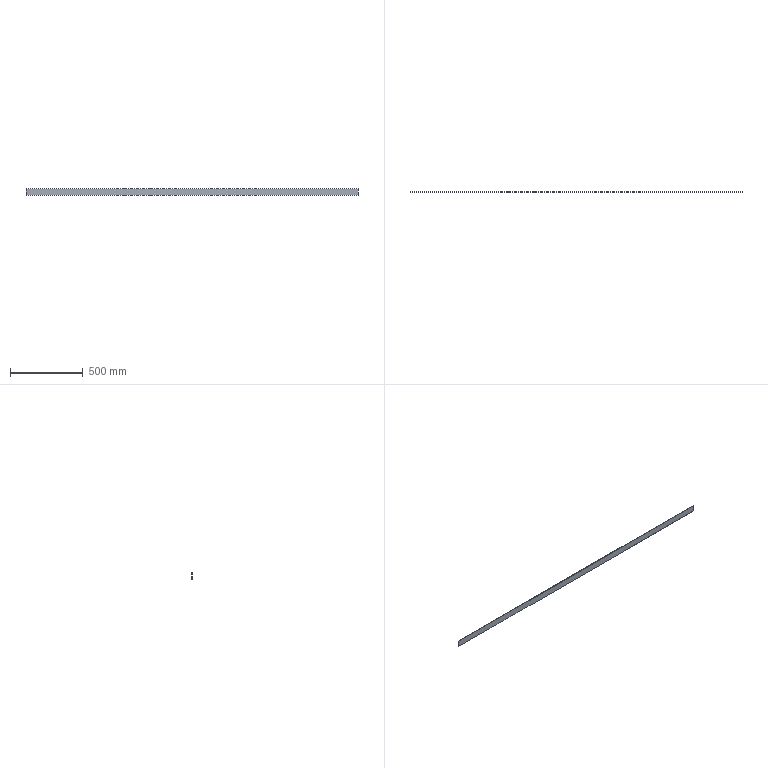Part | STEP file | SN10_017_003-01_CHAPA | 1 solid | 6 faces | box 2283 x 3 x 45 mm | volume 308205 mm3 | plane 6
STEP:
#1=CARTESIAN_POINT('',(0.,0.,0.));
#2=DIRECTION('',(0.,0.,1.));
#3=DIRECTION('',(1.,0.,0.));
#4=AXIS2_PLACEMENT_3D('',#1,#2,#3);
#5=CARTESIAN_POINT('',(3520.,-1740.,50.));
#6=VERTEX_POINT('',#5);
#7=CARTESIAN_POINT('',(1237.,-1740.,50.));
#8=VERTEX_POINT('',#7);
#9=CARTESIAN_POINT('',(3520.,-1740.,50.));
#10=DIRECTION('',(-1.,0.,0.));
#11=VECTOR('',#10,1.);
#12=LINE('',#9,#11);
#13=CARTESIAN_POINT('',(3520.,-1740.,95.));
#14=DIRECTION('',(0.,-1.,0.));
#15=DIRECTION('',(0.,0.,-1.));
#16=AXIS2_PLACEMENT_3D('',#13,#14,#15);
#17=PLANE('',#16);
#18=CARTESIAN_POINT('',(45.,0.));
#19=DIRECTION('',(0.,-1.));
#20=VECTOR('',#19,1.);
#21=LINE('',#18,#20);
#22=(GEOMETRIC_REPRESENTATION_CONTEXT(2)PARAMETRIC_REPRESENTATION_CONTEXT()REPRESENTATION_CONTEXT('',''));
#23=DEFINITIONAL_REPRESENTATION('',(#21),#22);
#24=PCURVE('',#17,#23);
#25=CARTESIAN_POINT('',(0.,0.,50.));
#26=DIRECTION('',(0.,0.,1.));
#27=DIRECTION('',(1.,0.,0.));
#28=AXIS2_PLACEMENT_3D('',#25,#26,#27);
#29=PLANE('',#28);
#30=CARTESIAN_POINT('',(3520.,-1740.));
#31=DIRECTION('',(-1.,0.));
#32=VECTOR('',#31,1.);
#33=LINE('',#30,#32);
#34=(GEOMETRIC_REPRESENTATION_CONTEXT(2)PARAMETRIC_REPRESENTATION_CONTEXT()REPRESENTATION_CONTEXT('',''));
#35=DEFINITIONAL_REPRESENTATION('',(#33),#34);
#36=PCURVE('',#29,#35);
#37=SURFACE_CURVE('',#12,(#24,#36),.PCURVE_S1.);
#38=EDGE_CURVE('',#6,#8,#37,.T.);
#39=ORIENTED_EDGE('',*,*,#38,.T.);
#40=CARTESIAN_POINT('',(1237.,-1740.,95.));
#41=VERTEX_POINT('',#40);
#42=CARTESIAN_POINT('',(1237.,-1740.,95.));
#43=DIRECTION('',(0.,0.,-1.));
#44=VECTOR('',#43,1.);
#45=LINE('',#42,#44);
#46=CARTESIAN_POINT('',(0.,-2283.));
#47=DIRECTION('',(1.,0.));
#48=VECTOR('',#47,1.);
#49=LINE('',#46,#48);
#50=(GEOMETRIC_REPRESENTATION_CONTEXT(2)PARAMETRIC_REPRESENTATION_CONTEXT()REPRESENTATION_CONTEXT('',''));
#51=DEFINITIONAL_REPRESENTATION('',(#49),#50);
#52=PCURVE('',#17,#51);
#53=CARTESIAN_POINT('',(1237.,-1740.,95.));
#54=DIRECTION('',(1.,0.,0.));
#55=DIRECTION('',(0.,0.,-1.));
#56=AXIS2_PLACEMENT_3D('',#53,#54,#55);
#57=PLANE('',#56);
#58=CARTESIAN_POINT('',(0.,0.));
#59=DIRECTION('',(1.,0.));
#60=VECTOR('',#59,1.);
#61=LINE('',#58,#60);
#62=(GEOMETRIC_REPRESENTATION_CONTEXT(2)PARAMETRIC_REPRESENTATION_CONTEXT()REPRESENTATION_CONTEXT('',''));
#63=DEFINITIONAL_REPRESENTATION('',(#61),#62);
#64=PCURVE('',#57,#63);
#65=SURFACE_CURVE('',#45,(#52,#64),.PCURVE_S1.);
#66=EDGE_CURVE('',#41,#8,#65,.T.);
#67=ORIENTED_EDGE('',*,*,#66,.F.);
#68=CARTESIAN_POINT('',(3520.,-1740.,95.));
#69=VERTEX_POINT('',#68);
#70=CARTESIAN_POINT('',(3520.,-1740.,95.));
#71=DIRECTION('',(-1.,0.,0.));
#72=VECTOR('',#71,1.);
#73=LINE('',#70,#72);
#74=CARTESIAN_POINT('',(0.,0.));
#75=DIRECTION('',(0.,-1.));
#76=VECTOR('',#75,1.);
#77=LINE('',#74,#76);
#78=(GEOMETRIC_REPRESENTATION_CONTEXT(2)PARAMETRIC_REPRESENTATION_CONTEXT()REPRESENTATION_CONTEXT('',''));
#79=DEFINITIONAL_REPRESENTATION('',(#77),#78);
#80=PCURVE('',#17,#79);
#81=CARTESIAN_POINT('',(0.,0.,95.));
#82=DIRECTION('',(0.,0.,1.));
#83=DIRECTION('',(1.,0.,0.));
#84=AXIS2_PLACEMENT_3D('',#81,#82,#83);
#85=PLANE('',#84);
#86=CARTESIAN_POINT('',(3520.,-1740.));
#87=DIRECTION('',(-1.,0.));
#88=VECTOR('',#87,1.);
#89=LINE('',#86,#88);
#90=(GEOMETRIC_REPRESENTATION_CONTEXT(2)PARAMETRIC_REPRESENTATION_CONTEXT()REPRESENTATION_CONTEXT('',''));
#91=DEFINITIONAL_REPRESENTATION('',(#89),#90);
#92=PCURVE('',#85,#91);
#93=SURFACE_CURVE('',#73,(#80,#92),.PCURVE_S1.);
#94=EDGE_CURVE('',#69,#41,#93,.T.);
#95=ORIENTED_EDGE('',*,*,#94,.F.);
#96=CARTESIAN_POINT('',(3520.,-1740.,95.));
#97=DIRECTION('',(0.,0.,-1.));
#98=VECTOR('',#97,1.);
#99=LINE('',#96,#98);
#100=CARTESIAN_POINT('',(0.,0.));
#101=DIRECTION('',(1.,0.));
#102=VECTOR('',#101,1.);
#103=LINE('',#100,#102);
#104=(GEOMETRIC_REPRESENTATION_CONTEXT(2)PARAMETRIC_REPRESENTATION_CONTEXT()REPRESENTATION_CONTEXT('',''));
#105=DEFINITIONAL_REPRESENTATION('',(#103),#104);
#106=PCURVE('',#17,#105);
#107=CARTESIAN_POINT('',(3520.,-1743.,95.));
#108=DIRECTION('',(-1.,0.,0.));
#109=DIRECTION('',(0.,0.,1.));
#110=AXIS2_PLACEMENT_3D('',#107,#108,#109);
#111=PLANE('',#110);
#112=CARTESIAN_POINT('',(0.,3.));
#113=DIRECTION('',(-1.,0.));
#114=VECTOR('',#113,1.);
#115=LINE('',#112,#114);
#116=(GEOMETRIC_REPRESENTATION_CONTEXT(2)PARAMETRIC_REPRESENTATION_CONTEXT()REPRESENTATION_CONTEXT('',''));
#117=DEFINITIONAL_REPRESENTATION('',(#115),#116);
#118=PCURVE('',#111,#117);
#119=SURFACE_CURVE('',#99,(#106,#118),.PCURVE_S1.);
#120=EDGE_CURVE('',#69,#6,#119,.T.);
#121=ORIENTED_EDGE('',*,*,#120,.T.);
#122=EDGE_LOOP('',(#39,#67,#95,#121));
#123=FACE_BOUND('',#122,.T.);
#124=ADVANCED_FACE('',(#123),#17,.F.);
#125=CARTESIAN_POINT('',(1237.,-1743.,50.));
#126=VERTEX_POINT('',#125);
#127=CARTESIAN_POINT('',(1237.,-1740.,50.));
#128=DIRECTION('',(0.,-1.,0.));
#129=VECTOR('',#128,1.);
#130=LINE('',#127,#129);
#131=CARTESIAN_POINT('',(45.,0.));
#132=DIRECTION('',(0.,-1.));
#133=VECTOR('',#132,1.);
#134=LINE('',#131,#133);
#135=(GEOMETRIC_REPRESENTATION_CONTEXT(2)PARAMETRIC_REPRESENTATION_CONTEXT()REPRESENTATION_CONTEXT('',''));
#136=DEFINITIONAL_REPRESENTATION('',(#134),#135);
#137=PCURVE('',#57,#136);
#138=CARTESIAN_POINT('',(1237.,-1740.));
#139=DIRECTION('',(0.,-1.));
#140=VECTOR('',#139,1.);
#141=LINE('',#138,#140);
#142=(GEOMETRIC_REPRESENTATION_CONTEXT(2)PARAMETRIC_REPRESENTATION_CONTEXT()REPRESENTATION_CONTEXT('',''));
#143=DEFINITIONAL_REPRESENTATION('',(#141),#142);
#144=PCURVE('',#29,#143);
#145=SURFACE_CURVE('',#130,(#137,#144),.PCURVE_S1.);
#146=EDGE_CURVE('',#8,#126,#145,.T.);
#147=ORIENTED_EDGE('',*,*,#146,.T.);
#148=CARTESIAN_POINT('',(1237.,-1743.,95.));
#149=VERTEX_POINT('',#148);
#150=CARTESIAN_POINT('',(1237.,-1743.,95.));
#151=DIRECTION('',(0.,0.,-1.));
#152=VECTOR('',#151,1.);
#153=LINE('',#150,#152);
#154=CARTESIAN_POINT('',(0.,-3.));
#155=DIRECTION('',(1.,0.));
#156=VECTOR('',#155,1.);
#157=LINE('',#154,#156);
#158=(GEOMETRIC_REPRESENTATION_CONTEXT(2)PARAMETRIC_REPRESENTATION_CONTEXT()REPRESENTATION_CONTEXT('',''));
#159=DEFINITIONAL_REPRESENTATION('',(#157),#158);
#160=PCURVE('',#57,#159);
#161=CARTESIAN_POINT('',(3520.,-1743.,95.));
#162=DIRECTION('',(0.,-1.,0.));
#163=DIRECTION('',(0.,0.,-1.));
#164=AXIS2_PLACEMENT_3D('',#161,#162,#163);
#165=PLANE('',#164);
#166=CARTESIAN_POINT('',(0.,-2283.));
#167=DIRECTION('',(1.,0.));
#168=VECTOR('',#167,1.);
#169=LINE('',#166,#168);
#170=(GEOMETRIC_REPRESENTATION_CONTEXT(2)PARAMETRIC_REPRESENTATION_CONTEXT()REPRESENTATION_CONTEXT('',''));
#171=DEFINITIONAL_REPRESENTATION('',(#169),#170);
#172=PCURVE('',#165,#171);
#173=SURFACE_CURVE('',#153,(#160,#172),.PCURVE_S1.);
#174=EDGE_CURVE('',#149,#126,#173,.T.);
#175=ORIENTED_EDGE('',*,*,#174,.F.);
#176=CARTESIAN_POINT('',(1237.,-1740.,95.));
#177=DIRECTION('',(0.,-1.,0.));
#178=VECTOR('',#177,1.);
#179=LINE('',#176,#178);
#180=CARTESIAN_POINT('',(0.,0.));
#181=DIRECTION('',(0.,-1.));
#182=VECTOR('',#181,1.);
#183=LINE('',#180,#182);
#184=(GEOMETRIC_REPRESENTATION_CONTEXT(2)PARAMETRIC_REPRESENTATION_CONTEXT()REPRESENTATION_CONTEXT('',''));
#185=DEFINITIONAL_REPRESENTATION('',(#183),#184);
#186=PCURVE('',#57,#185);
#187=CARTESIAN_POINT('',(1237.,-1740.));
#188=DIRECTION('',(0.,-1.));
#189=VECTOR('',#188,1.);
#190=LINE('',#187,#189);
#191=(GEOMETRIC_REPRESENTATION_CONTEXT(2)PARAMETRIC_REPRESENTATION_CONTEXT()REPRESENTATION_CONTEXT('',''));
#192=DEFINITIONAL_REPRESENTATION('',(#190),#191);
#193=PCURVE('',#85,#192);
#194=SURFACE_CURVE('',#179,(#186,#193),.PCURVE_S1.);
#195=EDGE_CURVE('',#41,#149,#194,.T.);
#196=ORIENTED_EDGE('',*,*,#195,.F.);
#197=ORIENTED_EDGE('',*,*,#66,.T.);
#198=EDGE_LOOP('',(#147,#175,#196,#197));
#199=FACE_BOUND('',#198,.T.);
#200=ADVANCED_FACE('',(#199),#57,.F.);
#201=CARTESIAN_POINT('',(3520.,-1743.,95.));
#202=VERTEX_POINT('',#201);
#203=CARTESIAN_POINT('',(3520.,-1743.,50.));
#204=VERTEX_POINT('',#203);
#205=CARTESIAN_POINT('',(3520.,-1743.,95.));
#206=DIRECTION('',(0.,0.,-1.));
#207=VECTOR('',#206,1.);
#208=LINE('',#205,#207);
#209=CARTESIAN_POINT('',(0.,0.));
#210=DIRECTION('',(1.,0.));
#211=VECTOR('',#210,1.);
#212=LINE('',#209,#211);
#213=(GEOMETRIC_REPRESENTATION_CONTEXT(2)PARAMETRIC_REPRESENTATION_CONTEXT()REPRESENTATION_CONTEXT('',''));
#214=DEFINITIONAL_REPRESENTATION('',(#212),#213);
#215=PCURVE('',#165,#214);
#216=CARTESIAN_POINT('',(0.,0.));
#217=DIRECTION('',(-1.,0.));
#218=VECTOR('',#217,1.);
#219=LINE('',#216,#218);
#220=(GEOMETRIC_REPRESENTATION_CONTEXT(2)PARAMETRIC_REPRESENTATION_CONTEXT()REPRESENTATION_CONTEXT('',''));
#221=DEFINITIONAL_REPRESENTATION('',(#219),#220);
#222=PCURVE('',#111,#221);
#223=SURFACE_CURVE('',#208,(#215,#222),.PCURVE_S1.);
#224=EDGE_CURVE('',#202,#204,#223,.T.);
#225=ORIENTED_EDGE('',*,*,#224,.F.);
#226=CARTESIAN_POINT('',(3520.,-1743.,95.));
#227=DIRECTION('',(-1.,0.,0.));
#228=VECTOR('',#227,1.);
#229=LINE('',#226,#228);
#230=CARTESIAN_POINT('',(0.,0.));
#231=DIRECTION('',(0.,-1.));
#232=VECTOR('',#231,1.);
#233=LINE('',#230,#232);
#234=(GEOMETRIC_REPRESENTATION_CONTEXT(2)PARAMETRIC_REPRESENTATION_CONTEXT()REPRESENTATION_CONTEXT('',''));
#235=DEFINITIONAL_REPRESENTATION('',(#233),#234);
#236=PCURVE('',#165,#235);
#237=CARTESIAN_POINT('',(3520.,-1743.));
#238=DIRECTION('',(-1.,0.));
#239=VECTOR('',#238,1.);
#240=LINE('',#237,#239);
#241=(GEOMETRIC_REPRESENTATION_CONTEXT(2)PARAMETRIC_REPRESENTATION_CONTEXT()REPRESENTATION_CONTEXT('',''));
#242=DEFINITIONAL_REPRESENTATION('',(#240),#241);
#243=PCURVE('',#85,#242);
#244=SURFACE_CURVE('',#229,(#236,#243),.PCURVE_S1.);
#245=EDGE_CURVE('',#202,#149,#244,.T.);
#246=ORIENTED_EDGE('',*,*,#245,.T.);
#247=ORIENTED_EDGE('',*,*,#174,.T.);
#248=CARTESIAN_POINT('',(3520.,-1743.,50.));
#249=DIRECTION('',(-1.,0.,0.));
#250=VECTOR('',#249,1.);
#251=LINE('',#248,#250);
#252=CARTESIAN_POINT('',(45.,0.));
#253=DIRECTION('',(0.,-1.));
#254=VECTOR('',#253,1.);
#255=LINE('',#252,#254);
#256=(GEOMETRIC_REPRESENTATION_CONTEXT(2)PARAMETRIC_REPRESENTATION_CONTEXT()REPRESENTATION_CONTEXT('',''));
#257=DEFINITIONAL_REPRESENTATION('',(#255),#256);
#258=PCURVE('',#165,#257);
#259=CARTESIAN_POINT('',(3520.,-1743.));
#260=DIRECTION('',(-1.,0.));
#261=VECTOR('',#260,1.);
#262=LINE('',#259,#261);
#263=(GEOMETRIC_REPRESENTATION_CONTEXT(2)PARAMETRIC_REPRESENTATION_CONTEXT()REPRESENTATION_CONTEXT('',''));
#264=DEFINITIONAL_REPRESENTATION('',(#262),#263);
#265=PCURVE('',#29,#264);
#266=SURFACE_CURVE('',#251,(#258,#265),.PCURVE_S1.);
#267=EDGE_CURVE('',#204,#126,#266,.T.);
#268=ORIENTED_EDGE('',*,*,#267,.F.);
#269=EDGE_LOOP('',(#225,#246,#247,#268));
#270=FACE_BOUND('',#269,.T.);
#271=ADVANCED_FACE('',(#270),#165,.T.);
#272=CARTESIAN_POINT('',(3520.,-1743.,50.));
#273=DIRECTION('',(0.,1.,0.));
#274=VECTOR('',#273,1.);
#275=LINE('',#272,#274);
#276=CARTESIAN_POINT('',(-45.,0.));
#277=DIRECTION('',(0.,1.));
#278=VECTOR('',#277,1.);
#279=LINE('',#276,#278);
#280=(GEOMETRIC_REPRESENTATION_CONTEXT(2)PARAMETRIC_REPRESENTATION_CONTEXT()REPRESENTATION_CONTEXT('',''));
#281=DEFINITIONAL_REPRESENTATION('',(#279),#280);
#282=PCURVE('',#111,#281);
#283=CARTESIAN_POINT('',(3520.,-1743.));
#284=DIRECTION('',(0.,1.));
#285=VECTOR('',#284,1.);
#286=LINE('',#283,#285);
#287=(GEOMETRIC_REPRESENTATION_CONTEXT(2)PARAMETRIC_REPRESENTATION_CONTEXT()REPRESENTATION_CONTEXT('',''));
#288=DEFINITIONAL_REPRESENTATION('',(#286),#287);
#289=PCURVE('',#29,#288);
#290=SURFACE_CURVE('',#275,(#282,#289),.PCURVE_S1.);
#291=EDGE_CURVE('',#204,#6,#290,.T.);
#292=ORIENTED_EDGE('',*,*,#291,.T.);
#293=ORIENTED_EDGE('',*,*,#120,.F.);
#294=CARTESIAN_POINT('',(3520.,-1743.,95.));
#295=DIRECTION('',(0.,1.,0.));
#296=VECTOR('',#295,1.);
#297=LINE('',#294,#296);
#298=CARTESIAN_POINT('',(0.,0.));
#299=DIRECTION('',(0.,1.));
#300=VECTOR('',#299,1.);
#301=LINE('',#298,#300);
#302=(GEOMETRIC_REPRESENTATION_CONTEXT(2)PARAMETRIC_REPRESENTATION_CONTEXT()REPRESENTATION_CONTEXT('',''));
#303=DEFINITIONAL_REPRESENTATION('',(#301),#302);
#304=PCURVE('',#111,#303);
#305=CARTESIAN_POINT('',(3520.,-1743.));
#306=DIRECTION('',(0.,1.));
#307=VECTOR('',#306,1.);
#308=LINE('',#305,#307);
#309=(GEOMETRIC_REPRESENTATION_CONTEXT(2)PARAMETRIC_REPRESENTATION_CONTEXT()REPRESENTATION_CONTEXT('',''));
#310=DEFINITIONAL_REPRESENTATION('',(#308),#309);
#311=PCURVE('',#85,#310);
#312=SURFACE_CURVE('',#297,(#304,#311),.PCURVE_S1.);
#313=EDGE_CURVE('',#202,#69,#312,.T.);
#314=ORIENTED_EDGE('',*,*,#313,.F.);
#315=ORIENTED_EDGE('',*,*,#224,.T.);
#316=EDGE_LOOP('',(#292,#293,#314,#315));
#317=FACE_BOUND('',#316,.T.);
#318=ADVANCED_FACE('',(#317),#111,.F.);
#319=ORIENTED_EDGE('',*,*,#94,.T.);
#320=ORIENTED_EDGE('',*,*,#195,.T.);
#321=ORIENTED_EDGE('',*,*,#245,.F.);
#322=ORIENTED_EDGE('',*,*,#313,.T.);
#323=EDGE_LOOP('',(#319,#320,#321,#322));
#324=FACE_BOUND('',#323,.T.);
#325=ADVANCED_FACE('',(#324),#85,.T.);
#326=ORIENTED_EDGE('',*,*,#291,.F.);
#327=ORIENTED_EDGE('',*,*,#267,.T.);
#328=ORIENTED_EDGE('',*,*,#146,.F.);
#329=ORIENTED_EDGE('',*,*,#38,.F.);
#330=EDGE_LOOP('',(#326,#327,#328,#329));
#331=FACE_BOUND('',#330,.T.);
#332=ADVANCED_FACE('',(#331),#29,.F.);
#333=CLOSED_SHELL('',(#124,#200,#271,#318,#325,#332));
#334=MANIFOLD_SOLID_BREP('',#333);
#335=(LENGTH_UNIT()NAMED_UNIT(*)SI_UNIT(.MILLI.,.METRE.));
#336=UNCERTAINTY_MEASURE_WITH_UNIT(LENGTH_MEASURE(0.0000001),#335,'','');
#337=(NAMED_UNIT(*)PLANE_ANGLE_UNIT()SI_UNIT($,.RADIAN.));
#338=(NAMED_UNIT(*)SI_UNIT($,.STERADIAN.)SOLID_ANGLE_UNIT());
#339=(GEOMETRIC_REPRESENTATION_CONTEXT(3)GLOBAL_UNCERTAINTY_ASSIGNED_CONTEXT((#336))GLOBAL_UNIT_ASSIGNED_CONTEXT((#335,#337,#338))REPRESENTATION_CONTEXT('',''));
#340=ADVANCED_BREP_SHAPE_REPRESENTATION('',(#4,#334),#339);